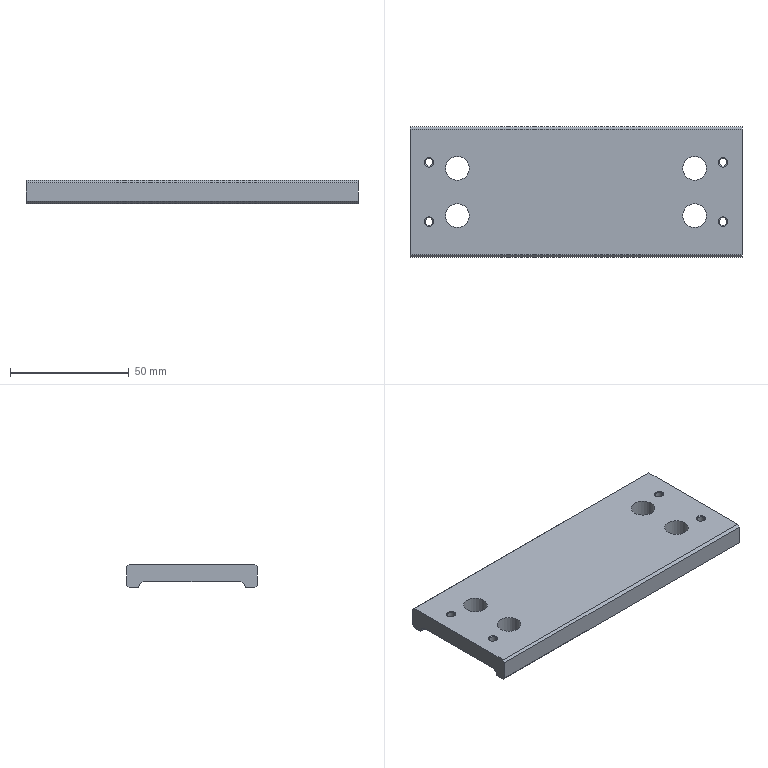Part | STEP file | Tube necking machine_id78_x_t | 1 solid | 30 faces | box 140 x 55 x 10 mm | volume 58090 mm3 | plane 12 | cylinder 10 | cone 8 | commonest cylinder face diameters 3.3 x4 10 x4 5.2 x2